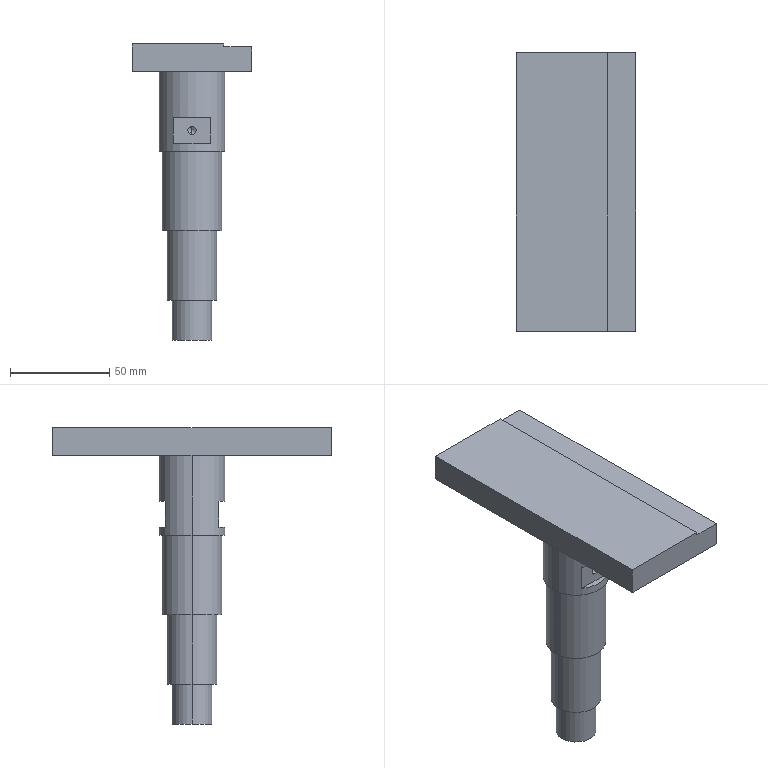Part | SolidWorks | features ICE 6, MirrorPattern 2, 3DProfileFeature 1, Extrusion 1, HoleWzd 1 | 1 solid | 34 faces | box 60 x 140 x 149 mm | volume 199315 mm3 | plane 18 | cylinder 12 | cone 4 | commonest cylinder face diameters 4.2 x4 20 x2 25 x2 30 x2 33 x2
STEP:
#1=CARTESIAN_POINT('',(0.,-3.5,52.6));
#2=VERTEX_POINT('',#1);
#3=CARTESIAN_POINT('',(0.,-3.5,48.4));
#4=VERTEX_POINT('',#3);
#5=CARTESIAN_POINT('',(0.,-3.5,50.5));
#6=DIRECTION('',(0.,-1.,0.));
#7=DIRECTION('',(0.,0.,-1.));
#8=AXIS2_PLACEMENT_3D('',#5,#6,#7);
#9=CIRCLE('',#8,2.1);
#10=EDGE_CURVE('',#2,#4,#9,.T.);
#11=ORIENTED_EDGE('',*,*,#10,.F.);
#12=CARTESIAN_POINT('',(0.,-13.5,52.6));
#13=VERTEX_POINT('',#12);
#14=CARTESIAN_POINT('',(0.,-13.5,52.6));
#15=DIRECTION('',(0.,-1.,0.));
#16=VECTOR('',#15,1000.);
#17=LINE('',#14,#16);
#18=EDGE_CURVE('',#2,#13,#17,.T.);
#19=ORIENTED_EDGE('',*,*,#18,.T.);
#20=CARTESIAN_POINT('',(0.,-13.5,48.4));
#21=VERTEX_POINT('',#20);
#22=CARTESIAN_POINT('',(0.,-13.5,50.5));
#23=DIRECTION('',(0.,-1.,0.));
#24=DIRECTION('',(0.,0.,-1.));
#25=AXIS2_PLACEMENT_3D('',#22,#23,#24);
#26=CIRCLE('',#25,2.1);
#27=EDGE_CURVE('',#13,#21,#26,.T.);
#28=ORIENTED_EDGE('',*,*,#27,.T.);
#29=CARTESIAN_POINT('',(0.,-13.5,48.4));
#30=DIRECTION('',(0.,-1.,0.));
#31=VECTOR('',#30,1000.);
#32=LINE('',#29,#31);
#33=EDGE_CURVE('',#4,#21,#32,.T.);
#34=ORIENTED_EDGE('',*,*,#33,.F.);
#35=EDGE_LOOP('',(#11,#19,#28,#34));
#36=FACE_OUTER_BOUND('',#35,.T.);
#37=CARTESIAN_POINT('',(0.,-13.5,50.5));
#38=DIRECTION('',(0.,-1.,0.));
#39=DIRECTION('',(0.,0.,-1.));
#40=AXIS2_PLACEMENT_3D('',#37,#38,#39);
#41=CYLINDRICAL_SURFACE('',#40,2.1);
#42=ADVANCED_FACE('',(#36),#41,.F.);
#43=CARTESIAN_POINT('',(0.,-2.238,50.5));
#44=VERTEX_POINT('',#43);
#45=CARTESIAN_POINT('',(0.,-3.5,48.4));
#46=DIRECTION('',(0.,-0.515,-0.8572));
#47=VECTOR('',#46,1000.);
#48=LINE('',#45,#47);
#49=EDGE_CURVE('',#44,#4,#48,.T.);
#50=ORIENTED_EDGE('',*,*,#49,.F.);
#51=CARTESIAN_POINT('',(0.,-3.5,52.6));
#52=DIRECTION('',(0.,-0.515,0.8572));
#53=VECTOR('',#52,1000.);
#54=LINE('',#51,#53);
#55=EDGE_CURVE('',#44,#2,#54,.T.);
#56=ORIENTED_EDGE('',*,*,#55,.T.);
#57=ORIENTED_EDGE('',*,*,#10,.T.);
#58=EDGE_LOOP('',(#50,#56,#57));
#59=FACE_OUTER_BOUND('',#58,.T.);
#60=CARTESIAN_POINT('',(0.,-3.5,50.5));
#61=DIRECTION('',(0.,-1.,0.));
#62=DIRECTION('',(0.,0.,-1.));
#63=AXIS2_PLACEMENT_3D('',#60,#61,#62);
#64=CONICAL_SURFACE('',#63,2.1,1.03);
#65=ADVANCED_FACE('',(#59),#64,.F.);
#66=CARTESIAN_POINT('',(0.,3.5,48.4));
#67=VERTEX_POINT('',#66);
#68=CARTESIAN_POINT('',(0.,3.5,52.6));
#69=VERTEX_POINT('',#68);
#70=CARTESIAN_POINT('',(0.,3.5,50.5));
#71=DIRECTION('',(0.,1.,0.));
#72=DIRECTION('',(0.,0.,1.));
#73=AXIS2_PLACEMENT_3D('',#70,#71,#72);
#74=CIRCLE('',#73,2.1);
#75=EDGE_CURVE('',#67,#69,#74,.T.);
#76=ORIENTED_EDGE('',*,*,#75,.F.);
#77=CARTESIAN_POINT('',(0.,13.5,48.4));
#78=VERTEX_POINT('',#77);
#79=CARTESIAN_POINT('',(0.,13.5,48.4));
#80=DIRECTION('',(0.,1.,0.));
#81=VECTOR('',#80,1000.);
#82=LINE('',#79,#81);
#83=EDGE_CURVE('',#67,#78,#82,.T.);
#84=ORIENTED_EDGE('',*,*,#83,.T.);
#85=CARTESIAN_POINT('',(0.,13.5,52.6));
#86=VERTEX_POINT('',#85);
#87=CARTESIAN_POINT('',(0.,13.5,50.5));
#88=DIRECTION('',(0.,1.,0.));
#89=DIRECTION('',(0.,0.,1.));
#90=AXIS2_PLACEMENT_3D('',#87,#88,#89);
#91=CIRCLE('',#90,2.1);
#92=EDGE_CURVE('',#78,#86,#91,.T.);
#93=ORIENTED_EDGE('',*,*,#92,.T.);
#94=CARTESIAN_POINT('',(0.,13.5,52.6));
#95=DIRECTION('',(0.,1.,0.));
#96=VECTOR('',#95,1000.);
#97=LINE('',#94,#96);
#98=EDGE_CURVE('',#69,#86,#97,.T.);
#99=ORIENTED_EDGE('',*,*,#98,.F.);
#100=EDGE_LOOP('',(#76,#84,#93,#99));
#101=FACE_OUTER_BOUND('',#100,.T.);
#102=CARTESIAN_POINT('',(0.,13.5,50.5));
#103=DIRECTION('',(0.,1.,0.));
#104=DIRECTION('',(0.,0.,1.));
#105=AXIS2_PLACEMENT_3D('',#102,#103,#104);
#106=CYLINDRICAL_SURFACE('',#105,2.1);
#107=ADVANCED_FACE('',(#101),#106,.F.);
#108=CARTESIAN_POINT('',(0.,2.238,50.5));
#109=VERTEX_POINT('',#108);
#110=CARTESIAN_POINT('',(0.,3.5,52.6));
#111=DIRECTION('',(0.,0.515,0.8572));
#112=VECTOR('',#111,1000.);
#113=LINE('',#110,#112);
#114=EDGE_CURVE('',#109,#69,#113,.T.);
#115=ORIENTED_EDGE('',*,*,#114,.F.);
#116=CARTESIAN_POINT('',(0.,3.5,48.4));
#117=DIRECTION('',(0.,0.515,-0.8572));
#118=VECTOR('',#117,1000.);
#119=LINE('',#116,#118);
#120=EDGE_CURVE('',#109,#67,#119,.T.);
#121=ORIENTED_EDGE('',*,*,#120,.T.);
#122=ORIENTED_EDGE('',*,*,#75,.T.);
#123=EDGE_LOOP('',(#115,#121,#122));
#124=FACE_OUTER_BOUND('',#123,.T.);
#125=CARTESIAN_POINT('',(0.,3.5,50.5));
#126=DIRECTION('',(0.,1.,0.));
#127=DIRECTION('',(0.,0.,1.));
#128=AXIS2_PLACEMENT_3D('',#125,#126,#127);
#129=CONICAL_SURFACE('',#128,2.1,1.03);
#130=ADVANCED_FACE('',(#124),#129,.F.);
#131=CARTESIAN_POINT('',(-10.,0.,-55.));
#132=VERTEX_POINT('',#131);
#133=CARTESIAN_POINT('',(10.,0.,-55.));
#134=VERTEX_POINT('',#133);
#135=CARTESIAN_POINT('',(0.,0.,-55.));
#136=DIRECTION('',(0.,0.,-1.));
#137=DIRECTION('',(-1.,0.,0.));
#138=AXIS2_PLACEMENT_3D('',#135,#136,#137);
#139=CIRCLE('',#138,10.);
#140=EDGE_CURVE('',#132,#134,#139,.T.);
#141=ORIENTED_EDGE('',*,*,#140,.F.);
#142=CARTESIAN_POINT('',(-10.,0.,-35.));
#143=VERTEX_POINT('',#142);
#144=CARTESIAN_POINT('',(-10.,0.,-55.));
#145=DIRECTION('',(0.,0.,1.));
#146=VECTOR('',#145,1000.);
#147=LINE('',#144,#146);
#148=EDGE_CURVE('',#132,#143,#147,.T.);
#149=ORIENTED_EDGE('',*,*,#148,.T.);
#150=CARTESIAN_POINT('',(10.,0.,-35.));
#151=VERTEX_POINT('',#150);
#152=CARTESIAN_POINT('',(0.,0.,-35.));
#153=DIRECTION('',(0.,0.,-1.));
#154=DIRECTION('',(-1.,0.,0.));
#155=AXIS2_PLACEMENT_3D('',#152,#153,#154);
#156=CIRCLE('',#155,10.);
#157=EDGE_CURVE('',#143,#151,#156,.T.);
#158=ORIENTED_EDGE('',*,*,#157,.T.);
#159=CARTESIAN_POINT('',(10.,0.,-55.));
#160=DIRECTION('',(0.,0.,1.));
#161=VECTOR('',#160,1000.);
#162=LINE('',#159,#161);
#163=EDGE_CURVE('',#134,#151,#162,.T.);
#164=ORIENTED_EDGE('',*,*,#163,.F.);
#165=EDGE_LOOP('',(#141,#149,#158,#164));
#166=FACE_OUTER_BOUND('',#165,.T.);
#167=CARTESIAN_POINT('',(0.,0.,-55.));
#168=DIRECTION('',(0.,0.,1.));
#169=DIRECTION('',(1.,0.,0.));
#170=AXIS2_PLACEMENT_3D('',#167,#168,#169);
#171=CYLINDRICAL_SURFACE('',#170,10.);
#172=ADVANCED_FACE('',(#166),#171,.T.);
#173=CARTESIAN_POINT('',(-12.5,0.,-35.));
#174=VERTEX_POINT('',#173);
#175=CARTESIAN_POINT('',(12.5,0.,-35.));
#176=VERTEX_POINT('',#175);
#177=CARTESIAN_POINT('',(0.,0.,-35.));
#178=DIRECTION('',(0.,0.,-1.));
#179=DIRECTION('',(-1.,0.,0.));
#180=AXIS2_PLACEMENT_3D('',#177,#178,#179);
#181=CIRCLE('',#180,12.5);
#182=EDGE_CURVE('',#174,#176,#181,.T.);
#183=ORIENTED_EDGE('',*,*,#182,.F.);
#184=CARTESIAN_POINT('',(-12.5,0.,0.));
#185=VERTEX_POINT('',#184);
#186=CARTESIAN_POINT('',(-12.5,0.,-35.));
#187=DIRECTION('',(0.,0.,1.));
#188=VECTOR('',#187,1000.);
#189=LINE('',#186,#188);
#190=EDGE_CURVE('',#174,#185,#189,.T.);
#191=ORIENTED_EDGE('',*,*,#190,.T.);
#192=CARTESIAN_POINT('',(12.5,0.,0.));
#193=VERTEX_POINT('',#192);
#194=CARTESIAN_POINT('',(0.,0.,0.));
#195=DIRECTION('',(0.,0.,-1.));
#196=DIRECTION('',(-1.,0.,0.));
#197=AXIS2_PLACEMENT_3D('',#194,#195,#196);
#198=CIRCLE('',#197,12.5);
#199=EDGE_CURVE('',#185,#193,#198,.T.);
#200=ORIENTED_EDGE('',*,*,#199,.T.);
#201=CARTESIAN_POINT('',(12.5,0.,-35.));
#202=DIRECTION('',(0.,0.,1.));
#203=VECTOR('',#202,1000.);
#204=LINE('',#201,#203);
#205=EDGE_CURVE('',#176,#193,#204,.T.);
#206=ORIENTED_EDGE('',*,*,#205,.F.);
#207=EDGE_LOOP('',(#183,#191,#200,#206));
#208=FACE_OUTER_BOUND('',#207,.T.);
#209=CARTESIAN_POINT('',(0.,0.,-35.));
#210=DIRECTION('',(0.,0.,1.));
#211=DIRECTION('',(1.,0.,0.));
#212=AXIS2_PLACEMENT_3D('',#209,#210,#211);
#213=CYLINDRICAL_SURFACE('',#212,12.5);
#214=ADVANCED_FACE('',(#208),#213,.T.);
#215=CARTESIAN_POINT('',(15.,0.,40.));
#216=VERTEX_POINT('',#215);
#217=CARTESIAN_POINT('',(-15.,0.,40.));
#218=VERTEX_POINT('',#217);
#219=CARTESIAN_POINT('',(0.,0.,40.));
#220=DIRECTION('',(0.,0.,1.));
#221=DIRECTION('',(1.,0.,0.));
#222=AXIS2_PLACEMENT_3D('',#219,#220,#221);
#223=CIRCLE('',#222,15.);
#224=EDGE_CURVE('',#216,#218,#223,.T.);
#225=ORIENTED_EDGE('',*,*,#224,.F.);
#226=CARTESIAN_POINT('',(15.,0.,0.));
#227=VERTEX_POINT('',#226);
#228=CARTESIAN_POINT('',(15.,0.,40.));
#229=DIRECTION('',(0.,0.,-1.));
#230=VECTOR('',#229,1000.);
#231=LINE('',#228,#230);
#232=EDGE_CURVE('',#216,#227,#231,.T.);
#233=ORIENTED_EDGE('',*,*,#232,.T.);
#234=CARTESIAN_POINT('',(-15.,0.,0.));
#235=VERTEX_POINT('',#234);
#236=CARTESIAN_POINT('',(0.,0.,0.));
#237=DIRECTION('',(0.,0.,1.));
#238=DIRECTION('',(1.,0.,0.));
#239=AXIS2_PLACEMENT_3D('',#236,#237,#238);
#240=CIRCLE('',#239,15.);
#241=EDGE_CURVE('',#227,#235,#240,.T.);
#242=ORIENTED_EDGE('',*,*,#241,.T.);
#243=CARTESIAN_POINT('',(-15.,0.,40.));
#244=DIRECTION('',(0.,0.,-1.));
#245=VECTOR('',#244,1000.);
#246=LINE('',#243,#245);
#247=EDGE_CURVE('',#218,#235,#246,.T.);
#248=ORIENTED_EDGE('',*,*,#247,.F.);
#249=EDGE_LOOP('',(#225,#233,#242,#248));
#250=FACE_OUTER_BOUND('',#249,.T.);
#251=CARTESIAN_POINT('',(0.,0.,40.));
#252=DIRECTION('',(0.,0.,-1.));
#253=DIRECTION('',(-1.,0.,0.));
#254=AXIS2_PLACEMENT_3D('',#251,#252,#253);
#255=CYLINDRICAL_SURFACE('',#254,15.);
#256=ADVANCED_FACE('',(#250),#255,.T.);
#257=CARTESIAN_POINT('',(-9.487,13.5,57.));
#258=VERTEX_POINT('',#257);
#259=CARTESIAN_POINT('',(-9.487,13.5,44.));
#260=VERTEX_POINT('',#259);
#261=CARTESIAN_POINT('',(-9.487,13.5,80.));
#262=DIRECTION('',(0.,0.,-1.));
#263=VECTOR('',#262,1000.);
#264=LINE('',#261,#263);
#265=EDGE_CURVE('',#258,#260,#264,.T.);
#266=ORIENTED_EDGE('',*,*,#265,.T.);
#267=CARTESIAN_POINT('',(9.487,13.5,44.));
#268=VERTEX_POINT('',#267);
#269=CARTESIAN_POINT('',(0.,0.,44.));
#270=DIRECTION('',(0.,0.,-1.));
#271=DIRECTION('',(-1.,0.,0.));
#272=AXIS2_PLACEMENT_3D('',#269,#270,#271);
#273=CIRCLE('',#272,16.5);
#274=EDGE_CURVE('',#260,#268,#273,.T.);
#275=ORIENTED_EDGE('',*,*,#274,.T.);
#276=CARTESIAN_POINT('',(9.487,13.5,57.));
#277=VERTEX_POINT('',#276);
#278=CARTESIAN_POINT('',(9.487,13.5,80.));
#279=DIRECTION('',(0.,0.,1.));
#280=VECTOR('',#279,1000.);
#281=LINE('',#278,#280);
#282=EDGE_CURVE('',#268,#277,#281,.T.);
#283=ORIENTED_EDGE('',*,*,#282,.T.);
#284=CARTESIAN_POINT('',(0.,0.,57.));
#285=DIRECTION('',(0.,0.,1.));
#286=DIRECTION('',(1.,0.,0.));
#287=AXIS2_PLACEMENT_3D('',#284,#285,#286);
#288=CIRCLE('',#287,16.5);
#289=EDGE_CURVE('',#277,#258,#288,.T.);
#290=ORIENTED_EDGE('',*,*,#289,.T.);
#291=EDGE_LOOP('',(#266,#275,#283,#290));
#292=FACE_BOUND('',#291,.T.);
#293=CARTESIAN_POINT('',(16.5,0.,80.));
#294=VERTEX_POINT('',#293);
#295=CARTESIAN_POINT('',(-16.5,0.,80.));
#296=VERTEX_POINT('',#295);
#297=CARTESIAN_POINT('',(0.,0.,80.));
#298=DIRECTION('',(0.,0.,1.));
#299=DIRECTION('',(1.,0.,0.));
#300=AXIS2_PLACEMENT_3D('',#297,#298,#299);
#301=CIRCLE('',#300,16.5);
#302=EDGE_CURVE('',#294,#296,#301,.T.);
#303=ORIENTED_EDGE('',*,*,#302,.F.);
#304=CARTESIAN_POINT('',(16.5,0.,40.));
#305=VERTEX_POINT('',#304);
#306=CARTESIAN_POINT('',(16.5,0.,80.));
#307=DIRECTION('',(0.,0.,-1.));
#308=VECTOR('',#307,1000.);
#309=LINE('',#306,#308);
#310=EDGE_CURVE('',#294,#305,#309,.T.);
#311=ORIENTED_EDGE('',*,*,#310,.T.);
#312=CARTESIAN_POINT('',(-16.5,0.,40.));
#313=VERTEX_POINT('',#312);
#314=CARTESIAN_POINT('',(0.,0.,40.));
#315=DIRECTION('',(0.,0.,1.));
#316=DIRECTION('',(1.,0.,0.));
#317=AXIS2_PLACEMENT_3D('',#314,#315,#316);
#318=CIRCLE('',#317,16.5);
#319=EDGE_CURVE('',#305,#313,#318,.T.);
#320=ORIENTED_EDGE('',*,*,#319,.T.);
#321=CARTESIAN_POINT('',(-16.5,0.,80.));
#322=DIRECTION('',(0.,0.,-1.));
#323=VECTOR('',#322,1000.);
#324=LINE('',#321,#323);
#325=EDGE_CURVE('',#296,#313,#324,.T.);
#326=ORIENTED_EDGE('',*,*,#325,.F.);
#327=EDGE_LOOP('',(#303,#311,#320,#326));
#328=FACE_OUTER_BOUND('',#327,.T.);
#329=CARTESIAN_POINT('',(0.,0.,80.));
#330=DIRECTION('',(0.,0.,-1.));
#331=DIRECTION('',(-1.,0.,0.));
#332=AXIS2_PLACEMENT_3D('',#329,#330,#331);
#333=CYLINDRICAL_SURFACE('',#332,16.5);
#334=ADVANCED_FACE('',(#292,#328),#333,.T.);
#335=ORIENTED_EDGE('',*,*,#310,.F.);
#336=CARTESIAN_POINT('',(0.,0.,80.));
#337=DIRECTION('',(0.,0.,1.));
#338=DIRECTION('',(1.,0.,0.));
#339=AXIS2_PLACEMENT_3D('',#336,#337,#338);
#340=CIRCLE('',#339,16.5);
#341=EDGE_CURVE('',#296,#294,#340,.T.);
#342=ORIENTED_EDGE('',*,*,#341,.F.);
#343=ORIENTED_EDGE('',*,*,#325,.T.);
#344=CARTESIAN_POINT('',(0.,0.,40.));
#345=DIRECTION('',(0.,0.,1.));
#346=DIRECTION('',(1.,0.,0.));
#347=AXIS2_PLACEMENT_3D('',#344,#345,#346);
#348=CIRCLE('',#347,16.5);
#349=EDGE_CURVE('',#313,#305,#348,.T.);
#350=ORIENTED_EDGE('',*,*,#349,.T.);
#351=EDGE_LOOP('',(#335,#342,#343,#350));
#352=FACE_OUTER_BOUND('',#351,.T.);
#353=CARTESIAN_POINT('',(9.487,-13.5,57.));
#354=VERTEX_POINT('',#353);
#355=CARTESIAN_POINT('',(-9.487,-13.5,57.));
#356=VERTEX_POINT('',#355);
#357=CARTESIAN_POINT('',(0.,0.,57.));
#358=DIRECTION('',(0.,0.,-1.));
#359=DIRECTION('',(-1.,0.,0.));
#360=AXIS2_PLACEMENT_3D('',#357,#358,#359);
#361=CIRCLE('',#360,16.5);
#362=EDGE_CURVE('',#354,#356,#361,.T.);
#363=ORIENTED_EDGE('',*,*,#362,.F.);
#364=CARTESIAN_POINT('',(9.487,-13.5,44.));
#365=VERTEX_POINT('',#364);
#366=CARTESIAN_POINT('',(9.487,-13.5,80.));
#367=DIRECTION('',(0.,0.,1.));
#368=VECTOR('',#367,1000.);
#369=LINE('',#366,#368);
#370=EDGE_CURVE('',#365,#354,#369,.T.);
#371=ORIENTED_EDGE('',*,*,#370,.F.);
#372=CARTESIAN_POINT('',(-9.487,-13.5,44.));
#373=VERTEX_POINT('',#372);
#374=CARTESIAN_POINT('',(0.,0.,44.));
#375=DIRECTION('',(0.,0.,1.));
#376=DIRECTION('',(1.,0.,0.));
#377=AXIS2_PLACEMENT_3D('',#374,#375,#376);
#378=CIRCLE('',#377,16.5);
#379=EDGE_CURVE('',#373,#365,#378,.T.);
#380=ORIENTED_EDGE('',*,*,#379,.F.);
#381=CARTESIAN_POINT('',(-9.487,-13.5,80.));
#382=DIRECTION('',(0.,0.,-1.));
#383=VECTOR('',#382,1000.);
#384=LINE('',#381,#383);
#385=EDGE_CURVE('',#356,#373,#384,.T.);
#386=ORIENTED_EDGE('',*,*,#385,.F.);
#387=EDGE_LOOP('',(#363,#371,#380,#386));
#388=FACE_BOUND('',#387,.T.);
#389=CARTESIAN_POINT('',(0.,0.,80.));
#390=DIRECTION('',(0.,0.,-1.));
#391=DIRECTION('',(-1.,0.,0.));
#392=AXIS2_PLACEMENT_3D('',#389,#390,#391);
#393=CYLINDRICAL_SURFACE('',#392,16.5);
#394=ADVANCED_FACE('',(#352,#388),#393,.T.);
#395=ORIENTED_EDGE('',*,*,#232,.F.);
#396=CARTESIAN_POINT('',(0.,0.,40.));
#397=DIRECTION('',(0.,0.,1.));
#398=DIRECTION('',(1.,0.,0.));
#399=AXIS2_PLACEMENT_3D('',#396,#397,#398);
#400=CIRCLE('',#399,15.);
#401=EDGE_CURVE('',#218,#216,#400,.T.);
#402=ORIENTED_EDGE('',*,*,#401,.F.);
#403=ORIENTED_EDGE('',*,*,#247,.T.);
#404=CARTESIAN_POINT('',(0.,0.,0.));
#405=DIRECTION('',(0.,0.,1.));
#406=DIRECTION('',(1.,0.,0.));
#407=AXIS2_PLACEMENT_3D('',#404,#405,#406);
#408=CIRCLE('',#407,15.);
#409=EDGE_CURVE('',#235,#227,#408,.T.);
#410=ORIENTED_EDGE('',*,*,#409,.T.);
#411=EDGE_LOOP('',(#395,#402,#403,#410));
#412=FACE_OUTER_BOUND('',#411,.T.);
#413=CARTESIAN_POINT('',(0.,0.,40.));
#414=DIRECTION('',(0.,0.,-1.));
#415=DIRECTION('',(-1.,0.,0.));
#416=AXIS2_PLACEMENT_3D('',#413,#414,#415);
#417=CYLINDRICAL_SURFACE('',#416,15.);
#418=ADVANCED_FACE('',(#412),#417,.T.);
#419=CARTESIAN_POINT('',(0.,0.,0.));
#420=DIRECTION('',(0.,0.,-1.));
#421=DIRECTION('',(-1.,0.,0.));
#422=AXIS2_PLACEMENT_3D('',#419,#420,#421);
#423=CIRCLE('',#422,12.5);
#424=EDGE_CURVE('',#193,#185,#423,.T.);
#425=ORIENTED_EDGE('',*,*,#424,.F.);
#426=ORIENTED_EDGE('',*,*,#199,.F.);
#427=EDGE_LOOP('',(#425,#426));
#428=FACE_BOUND('',#427,.T.);
#429=ORIENTED_EDGE('',*,*,#409,.F.);
#430=ORIENTED_EDGE('',*,*,#241,.F.);
#431=EDGE_LOOP('',(#429,#430));
#432=FACE_OUTER_BOUND('',#431,.T.);
#433=CARTESIAN_POINT('',(0.,0.,0.));
#434=DIRECTION('',(0.,0.,1.));
#435=DIRECTION('',(1.,0.,0.));
#436=AXIS2_PLACEMENT_3D('',#433,#434,#435);
#437=PLANE('',#436);
#438=ADVANCED_FACE('',(#428,#432),#437,.F.);
#439=ORIENTED_EDGE('',*,*,#401,.T.);
#440=ORIENTED_EDGE('',*,*,#224,.T.);
#441=EDGE_LOOP('',(#439,#440));
#442=FACE_BOUND('',#441,.T.);
#443=ORIENTED_EDGE('',*,*,#349,.F.);
#444=ORIENTED_EDGE('',*,*,#319,.F.);
#445=EDGE_LOOP('',(#443,#444));
#446=FACE_OUTER_BOUND('',#445,.T.);
#447=CARTESIAN_POINT('',(0.,0.,40.));
#448=DIRECTION('',(0.,0.,1.));
#449=DIRECTION('',(1.,0.,0.));
#450=AXIS2_PLACEMENT_3D('',#447,#448,#449);
#451=PLANE('',#450);
#452=ADVANCED_FACE('',(#442,#446),#451,.F.);
#453=ORIENTED_EDGE('',*,*,#190,.F.);
#454=CARTESIAN_POINT('',(0.,0.,-35.));
#455=DIRECTION('',(0.,0.,-1.));
#456=DIRECTION('',(-1.,0.,0.));
#457=AXIS2_PLACEMENT_3D('',#454,#455,#456);
#458=CIRCLE('',#457,12.5);
#459=EDGE_CURVE('',#176,#174,#458,.T.);
#460=ORIENTED_EDGE('',*,*,#459,.F.);
#461=ORIENTED_EDGE('',*,*,#205,.T.);
#462=ORIENTED_EDGE('',*,*,#424,.T.);
#463=EDGE_LOOP('',(#453,#460,#461,#462));
#464=FACE_OUTER_BOUND('',#463,.T.);
#465=CARTESIAN_POINT('',(0.,0.,-35.));
#466=DIRECTION('',(0.,0.,1.));
#467=DIRECTION('',(1.,0.,0.));
#468=AXIS2_PLACEMENT_3D('',#465,#466,#467);
#469=CYLINDRICAL_SURFACE('',#468,12.5);
#470=ADVANCED_FACE('',(#464),#469,.T.);
#471=CARTESIAN_POINT('',(0.,0.,-35.));
#472=DIRECTION('',(0.,0.,-1.));
#473=DIRECTION('',(-1.,0.,0.));
#474=AXIS2_PLACEMENT_3D('',#471,#472,#473);
#475=CIRCLE('',#474,10.);
#476=EDGE_CURVE('',#151,#143,#475,.T.);
#477=ORIENTED_EDGE('',*,*,#476,.F.);
#478=ORIENTED_EDGE('',*,*,#157,.F.);
#479=EDGE_LOOP('',(#477,#478));
#480=FACE_BOUND('',#479,.T.);
#481=ORIENTED_EDGE('',*,*,#459,.T.);
#482=ORIENTED_EDGE('',*,*,#182,.T.);
#483=EDGE_LOOP('',(#481,#482));
#484=FACE_OUTER_BOUND('',#483,.T.);
#485=CARTESIAN_POINT('',(0.,0.,-35.));
#486=DIRECTION('',(0.,0.,-1.));
#487=DIRECTION('',(-1.,0.,0.));
#488=AXIS2_PLACEMENT_3D('',#485,#486,#487);
#489=PLANE('',#488);
#490=ADVANCED_FACE('',(#480,#484),#489,.T.);
#491=ORIENTED_EDGE('',*,*,#148,.F.);
#492=CARTESIAN_POINT('',(0.,0.,-55.));
#493=DIRECTION('',(0.,0.,-1.));
#494=DIRECTION('',(-1.,0.,0.));
#495=AXIS2_PLACEMENT_3D('',#492,#493,#494);
#496=CIRCLE('',#495,10.);
#497=EDGE_CURVE('',#134,#132,#496,.T.);
#498=ORIENTED_EDGE('',*,*,#497,.F.);
#499=ORIENTED_EDGE('',*,*,#163,.T.);
#500=ORIENTED_EDGE('',*,*,#476,.T.);
#501=EDGE_LOOP('',(#491,#498,#499,#500));
#502=FACE_OUTER_BOUND('',#501,.T.);
#503=CARTESIAN_POINT('',(0.,0.,-55.));
#504=DIRECTION('',(0.,0.,1.));
#505=DIRECTION('',(1.,0.,0.));
#506=AXIS2_PLACEMENT_3D('',#503,#504,#505);
#507=CYLINDRICAL_SURFACE('',#506,10.);
#508=ADVANCED_FACE('',(#502),#507,.T.);
#509=ORIENTED_EDGE('',*,*,#497,.T.);
#510=ORIENTED_EDGE('',*,*,#140,.T.);
#511=EDGE_LOOP('',(#509,#510));
#512=FACE_OUTER_BOUND('',#511,.T.);
#513=CARTESIAN_POINT('',(0.,0.,-55.));
#514=DIRECTION('',(0.,0.,-1.));
#515=DIRECTION('',(-1.,0.,0.));
#516=AXIS2_PLACEMENT_3D('',#513,#514,#515);
#517=PLANE('',#516);
#518=ADVANCED_FACE('',(#512),#517,.T.);
#519=CARTESIAN_POINT('',(30.,70.,92.5));
#520=VERTEX_POINT('',#519);
#521=CARTESIAN_POINT('',(30.,70.,80.));
#522=VERTEX_POINT('',#521);
#523=CARTESIAN_POINT('',(30.,70.,94.));
#524=DIRECTION('',(0.,0.,-1.));
#525=VECTOR('',#524,1000.);
#526=LINE('',#523,#525);
#527=EDGE_CURVE('',#520,#522,#526,.T.);
#528=ORIENTED_EDGE('',*,*,#527,.F.);
#529=CARTESIAN_POINT('',(30.,-70.,92.5));
#530=VERTEX_POINT('',#529);
#531=CARTESIAN_POINT('',(30.,70.,92.5));
#532=DIRECTION('',(0.,1.,0.));
#533=VECTOR('',#532,1000.);
#534=LINE('',#531,#533);
#535=EDGE_CURVE('',#530,#520,#534,.T.);
#536=ORIENTED_EDGE('',*,*,#535,.F.);
#537=CARTESIAN_POINT('',(30.,-70.,80.));
#538=VERTEX_POINT('',#537);
#539=CARTESIAN_POINT('',(30.,-70.,94.));
#540=DIRECTION('',(0.,0.,-1.));
#541=VECTOR('',#540,1000.);
#542=LINE('',#539,#541);
#543=EDGE_CURVE('',#530,#538,#542,.T.);
#544=ORIENTED_EDGE('',*,*,#543,.T.);
#545=CARTESIAN_POINT('',(30.,-70.,80.));
#546=DIRECTION('',(0.,1.,0.));
#547=VECTOR('',#546,1000.);
#548=LINE('',#545,#547);
#549=EDGE_CURVE('',#538,#522,#548,.T.);
#550=ORIENTED_EDGE('',*,*,#549,.T.);
#551=EDGE_LOOP('',(#528,#536,#544,#550));
#552=FACE_OUTER_BOUND('',#551,.T.);
#553=CARTESIAN_POINT('',(30.,-70.,94.));
#554=DIRECTION('',(-1.,0.,0.));
#555=DIRECTION('',(0.,0.,1.));
#556=AXIS2_PLACEMENT_3D('',#553,#554,#555);
#557=PLANE('',#556);
#558=ADVANCED_FACE('',(#552),#557,.F.);
#559=CARTESIAN_POINT('',(16.,70.,94.));
#560=VERTEX_POINT('',#559);
#561=CARTESIAN_POINT('',(-30.,70.,94.));
#562=VERTEX_POINT('',#561);
#563=CARTESIAN_POINT('',(-30.,70.,94.));
#564=DIRECTION('',(-1.,0.,0.));
#565=VECTOR('',#564,1000.);
#566=LINE('',#563,#565);
#567=EDGE_CURVE('',#560,#562,#566,.T.);
#568=ORIENTED_EDGE('',*,*,#567,.F.);
#569=CARTESIAN_POINT('',(16.,70.,92.5));
#570=VERTEX_POINT('',#569);
#571=CARTESIAN_POINT('',(16.,70.,92.5));
#572=DIRECTION('',(0.,0.,1.));
#573=VECTOR('',#572,1000.);
#574=LINE('',#571,#573);
#575=EDGE_CURVE('',#570,#560,#574,.T.);
#576=ORIENTED_EDGE('',*,*,#575,.F.);
#577=CARTESIAN_POINT('',(30.,70.,92.5));
#578=DIRECTION('',(-1.,0.,0.));
#579=VECTOR('',#578,1000.);
#580=LINE('',#577,#579);
#581=EDGE_CURVE('',#520,#570,#580,.T.);
#582=ORIENTED_EDGE('',*,*,#581,.F.);
#583=ORIENTED_EDGE('',*,*,#527,.T.);
#584=CARTESIAN_POINT('',(-30.,70.,80.));
#585=VERTEX_POINT('',#584);
#586=CARTESIAN_POINT('',(-30.,70.,80.));
#587=DIRECTION('',(-1.,0.,0.));
#588=VECTOR('',#587,1000.);
#589=LINE('',#586,#588);
#590=EDGE_CURVE('',#522,#585,#589,.T.);
#591=ORIENTED_EDGE('',*,*,#590,.T.);
#592=CARTESIAN_POINT('',(-30.,70.,94.));
#593=DIRECTION('',(0.,0.,-1.));
#594=VECTOR('',#593,1000.);
#595=LINE('',#592,#594);
#596=EDGE_CURVE('',#562,#585,#595,.T.);
#597=ORIENTED_EDGE('',*,*,#596,.F.);
#598=EDGE_LOOP('',(#568,#576,#582,#583,#591,#597));
#599=FACE_OUTER_BOUND('',#598,.T.);
#600=CARTESIAN_POINT('',(-30.,70.,94.));
#601=DIRECTION('',(0.,-1.,0.));
#602=DIRECTION('',(0.,0.,-1.));
#603=AXIS2_PLACEMENT_3D('',#600,#601,#602);
#604=PLANE('',#603);
#605=ADVANCED_FACE('',(#599),#604,.F.);
#606=CARTESIAN_POINT('',(-30.,-70.,80.));
#607=VERTEX_POINT('',#606);
#608=CARTESIAN_POINT('',(-30.,-70.,80.));
#609=DIRECTION('',(0.,-1.,0.));
#610=VECTOR('',#609,1000.);
#611=LINE('',#608,#610);
#612=EDGE_CURVE('',#585,#607,#611,.T.);
#613=ORIENTED_EDGE('',*,*,#612,.T.);
#614=CARTESIAN_POINT('',(-30.,-70.,94.));
#615=VERTEX_POINT('',#614);
#616=CARTESIAN_POINT('',(-30.,-70.,94.));
#617=DIRECTION('',(0.,0.,-1.));
#618=VECTOR('',#617,1000.);
#619=LINE('',#616,#618);
#620=EDGE_CURVE('',#615,#607,#619,.T.);
#621=ORIENTED_EDGE('',*,*,#620,.F.);
#622=CARTESIAN_POINT('',(-30.,-70.,94.));
#623=DIRECTION('',(0.,-1.,0.));
#624=VECTOR('',#623,1000.);
#625=LINE('',#622,#624);
#626=EDGE_CURVE('',#562,#615,#625,.T.);
#627=ORIENTED_EDGE('',*,*,#626,.F.);
#628=ORIENTED_EDGE('',*,*,#596,.T.);
#629=EDGE_LOOP('',(#613,#621,#627,#628));
#630=FACE_OUTER_BOUND('',#629,.T.);
#631=CARTESIAN_POINT('',(-30.,-70.,94.));
#632=DIRECTION('',(1.,0.,0.));
#633=DIRECTION('',(0.,0.,-1.));
#634=AXIS2_PLACEMENT_3D('',#631,#632,#633);
#635=PLANE('',#634);
#636=ADVANCED_FACE('',(#630),#635,.F.);
#637=CARTESIAN_POINT('',(16.,-70.,92.5));
#638=VERTEX_POINT('',#637);
#639=CARTESIAN_POINT('',(30.,-70.,92.5));
#640=DIRECTION('',(1.,0.,0.));
#641=VECTOR('',#640,1000.);
#642=LINE('',#639,#641);
#643=EDGE_CURVE('',#638,#530,#642,.T.);
#644=ORIENTED_EDGE('',*,*,#643,.F.);
#645=CARTESIAN_POINT('',(16.,-70.,94.));
#646=VERTEX_POINT('',#645);
#647=CARTESIAN_POINT('',(16.,-70.,92.5));
#648=DIRECTION('',(0.,0.,1.));
#649=VECTOR('',#648,1000.);
#650=LINE('',#647,#649);
#651=EDGE_CURVE('',#638,#646,#650,.T.);
#652=ORIENTED_EDGE('',*,*,#651,.T.);
#653=CARTESIAN_POINT('',(-30.,-70.,94.));
#654=DIRECTION('',(1.,0.,0.));
#655=VECTOR('',#654,1000.);
#656=LINE('',#653,#655);
#657=EDGE_CURVE('',#615,#646,#656,.T.);
#658=ORIENTED_EDGE('',*,*,#657,.F.);
#659=ORIENTED_EDGE('',*,*,#620,.T.);
#660=CARTESIAN_POINT('',(-30.,-70.,80.));
#661=DIRECTION('',(1.,0.,0.));
#662=VECTOR('',#661,1000.);
#663=LINE('',#660,#662);
#664=EDGE_CURVE('',#607,#538,#663,.T.);
#665=ORIENTED_EDGE('',*,*,#664,.T.);
#666=ORIENTED_EDGE('',*,*,#543,.F.);
#667=EDGE_LOOP('',(#644,#652,#658,#659,#665,#666));
#668=FACE_OUTER_BOUND('',#667,.T.);
#669=CARTESIAN_POINT('',(-30.,-70.,94.));
#670=DIRECTION('',(0.,1.,0.));
#671=DIRECTION('',(0.,0.,1.));
#672=AXIS2_PLACEMENT_3D('',#669,#670,#671);
#673=PLANE('',#672);
#674=ADVANCED_FACE('',(#668),#673,.F.);
#675=ORIENTED_EDGE('',*,*,#657,.T.);
#676=CARTESIAN_POINT('',(16.,70.,94.));
#677=DIRECTION('',(0.,-1.,0.));
#678=VECTOR('',#677,1000.);
#679=LINE('',#676,#678);
#680=EDGE_CURVE('',#560,#646,#679,.T.);
#681=ORIENTED_EDGE('',*,*,#680,.F.);
#682=ORIENTED_EDGE('',*,*,#567,.T.);
#683=ORIENTED_EDGE('',*,*,#626,.T.);
#684=EDGE_LOOP('',(#675,#681,#682,#683));
#685=FACE_OUTER_BOUND('',#684,.T.);
#686=CARTESIAN_POINT('',(0.,0.,94.));
#687=DIRECTION('',(0.,0.,-1.));
#688=DIRECTION('',(-1.,0.,0.));
#689=AXIS2_PLACEMENT_3D('',#686,#687,#688);
#690=PLANE('',#689);
#691=ADVANCED_FACE('',(#685),#690,.F.);
#692=ORIENTED_EDGE('',*,*,#341,.T.);
#693=ORIENTED_EDGE('',*,*,#302,.T.);
#694=EDGE_LOOP('',(#692,#693));
#695=FACE_BOUND('',#694,.T.);
#696=ORIENTED_EDGE('',*,*,#549,.F.);
#697=ORIENTED_EDGE('',*,*,#664,.F.);
#698=ORIENTED_EDGE('',*,*,#612,.F.);
#699=ORIENTED_EDGE('',*,*,#590,.F.);
#700=EDGE_LOOP('',(#696,#697,#698,#699));
#701=FACE_OUTER_BOUND('',#700,.T.);
#702=CARTESIAN_POINT('',(0.,0.,80.));
#703=DIRECTION('',(0.,0.,-1.));
#704=DIRECTION('',(-1.,0.,0.));
#705=AXIS2_PLACEMENT_3D('',#702,#703,#704);
#706=PLANE('',#705);
#707=ADVANCED_FACE('',(#695,#701),#706,.T.);
#708=ORIENTED_EDGE('',*,*,#680,.T.);
#709=ORIENTED_EDGE('',*,*,#651,.F.);
#710=CARTESIAN_POINT('',(16.,70.,92.5));
#711=DIRECTION('',(0.,-1.,0.));
#712=VECTOR('',#711,1000.);
#713=LINE('',#710,#712);
#714=EDGE_CURVE('',#570,#638,#713,.T.);
#715=ORIENTED_EDGE('',*,*,#714,.F.);
#716=ORIENTED_EDGE('',*,*,#575,.T.);
#717=EDGE_LOOP('',(#708,#709,#715,#716));
#718=FACE_OUTER_BOUND('',#717,.T.);
#719=CARTESIAN_POINT('',(16.,70.,92.5));
#720=DIRECTION('',(-1.,0.,0.));
#721=DIRECTION('',(0.,-1.,0.));
#722=AXIS2_PLACEMENT_3D('',#719,#720,#721);
#723=PLANE('',#722);
#724=ADVANCED_FACE('',(#718),#723,.F.);
#725=ORIENTED_EDGE('',*,*,#535,.T.);
#726=ORIENTED_EDGE('',*,*,#581,.T.);
#727=ORIENTED_EDGE('',*,*,#714,.T.);
#728=ORIENTED_EDGE('',*,*,#643,.T.);
#729=EDGE_LOOP('',(#725,#726,#727,#728));
#730=FACE_OUTER_BOUND('',#729,.T.);
#731=CARTESIAN_POINT('',(0.,0.,92.5));
#732=DIRECTION('',(0.,0.,-1.));
#733=DIRECTION('',(-1.,0.,0.));
#734=AXIS2_PLACEMENT_3D('',#731,#732,#733);
#735=PLANE('',#734);
#736=ADVANCED_FACE('',(#730),#735,.F.);
#737=CARTESIAN_POINT('',(-10.,13.5,44.));
#738=DIRECTION('',(1.,0.,0.));
#739=VECTOR('',#738,1000.);
#740=LINE('',#737,#739);
#741=EDGE_CURVE('',#260,#268,#740,.T.);
#742=ORIENTED_EDGE('',*,*,#741,.T.);
#743=ORIENTED_EDGE('',*,*,#274,.F.);
#744=EDGE_LOOP('',(#742,#743));
#745=FACE_OUTER_BOUND('',#744,.T.);
#746=CARTESIAN_POINT('',(-10.,13.5,44.));
#747=DIRECTION('',(0.,0.,-1.));
#748=DIRECTION('',(-1.,0.,0.));
#749=AXIS2_PLACEMENT_3D('',#746,#747,#748);
#750=PLANE('',#749);
#751=ADVANCED_FACE('',(#745),#750,.F.);
#752=CARTESIAN_POINT('',(0.,13.5,50.5));
#753=DIRECTION('',(0.,1.,0.));
#754=DIRECTION('',(0.,0.,1.));
#755=AXIS2_PLACEMENT_3D('',#752,#753,#754);
#756=CIRCLE('',#755,2.1);
#757=EDGE_CURVE('',#86,#78,#756,.T.);
#758=ORIENTED_EDGE('',*,*,#757,.F.);
#759=ORIENTED_EDGE('',*,*,#92,.F.);
#760=EDGE_LOOP('',(#758,#759));
#761=FACE_BOUND('',#760,.T.);
#762=CARTESIAN_POINT('',(-10.,13.5,57.));
#763=DIRECTION('',(1.,0.,0.));
#764=VECTOR('',#763,1000.);
#765=LINE('',#762,#764);
#766=EDGE_CURVE('',#258,#277,#765,.T.);
#767=ORIENTED_EDGE('',*,*,#766,.T.);
#768=ORIENTED_EDGE('',*,*,#282,.F.);
#769=ORIENTED_EDGE('',*,*,#741,.F.);
#770=ORIENTED_EDGE('',*,*,#265,.F.);
#771=EDGE_LOOP('',(#767,#768,#769,#770));
#772=FACE_OUTER_BOUND('',#771,.T.);
#773=CARTESIAN_POINT('',(-10.,13.5,57.));
#774=DIRECTION('',(0.,-1.,0.));
#775=DIRECTION('',(0.,0.,-1.));
#776=AXIS2_PLACEMENT_3D('',#773,#774,#775);
#777=PLANE('',#776);
#778=ADVANCED_FACE('',(#761,#772),#777,.F.);
#779=ORIENTED_EDGE('',*,*,#766,.F.);
#780=ORIENTED_EDGE('',*,*,#289,.F.);
#781=EDGE_LOOP('',(#779,#780));
#782=FACE_OUTER_BOUND('',#781,.T.);
#783=CARTESIAN_POINT('',(-10.,16.5,57.));
#784=DIRECTION('',(0.,0.,1.));
#785=DIRECTION('',(1.,0.,0.));
#786=AXIS2_PLACEMENT_3D('',#783,#784,#785);
#787=PLANE('',#786);
#788=ADVANCED_FACE('',(#782),#787,.F.);
#789=CARTESIAN_POINT('',(-10.,-13.5,57.));
#790=DIRECTION('',(1.,0.,0.));
#791=VECTOR('',#790,1000.);
#792=LINE('',#789,#791);
#793=EDGE_CURVE('',#356,#354,#792,.T.);
#794=ORIENTED_EDGE('',*,*,#793,.T.);
#795=ORIENTED_EDGE('',*,*,#362,.T.);
#796=EDGE_LOOP('',(#794,#795));
#797=FACE_OUTER_BOUND('',#796,.T.);
#798=CARTESIAN_POINT('',(-10.,-16.5,57.));
#799=DIRECTION('',(0.,0.,-1.));
#800=DIRECTION('',(-1.,0.,0.));
#801=AXIS2_PLACEMENT_3D('',#798,#799,#800);
#802=PLANE('',#801);
#803=ADVANCED_FACE('',(#797),#802,.T.);
#804=CARTESIAN_POINT('',(0.,-13.5,50.5));
#805=DIRECTION('',(0.,-1.,0.));
#806=DIRECTION('',(0.,0.,-1.));
#807=AXIS2_PLACEMENT_3D('',#804,#805,#806);
#808=CIRCLE('',#807,2.1);
#809=EDGE_CURVE('',#21,#13,#808,.T.);
#810=ORIENTED_EDGE('',*,*,#809,.F.);
#811=ORIENTED_EDGE('',*,*,#27,.F.);
#812=EDGE_LOOP('',(#810,#811));
#813=FACE_BOUND('',#812,.T.);
#814=ORIENTED_EDGE('',*,*,#385,.T.);
#815=CARTESIAN_POINT('',(-10.,-13.5,44.));
#816=DIRECTION('',(1.,0.,0.));
#817=VECTOR('',#816,1000.);
#818=LINE('',#815,#817);
#819=EDGE_CURVE('',#373,#365,#818,.T.);
#820=ORIENTED_EDGE('',*,*,#819,.T.);
#821=ORIENTED_EDGE('',*,*,#370,.T.);
#822=ORIENTED_EDGE('',*,*,#793,.F.);
#823=EDGE_LOOP('',(#814,#820,#821,#822));
#824=FACE_OUTER_BOUND('',#823,.T.);
#825=CARTESIAN_POINT('',(-10.,-13.5,57.));
#826=DIRECTION('',(0.,-1.,0.));
#827=DIRECTION('',(0.,0.,-1.));
#828=AXIS2_PLACEMENT_3D('',#825,#826,#827);
#829=PLANE('',#828);
#830=ADVANCED_FACE('',(#813,#824),#829,.T.);
#831=ORIENTED_EDGE('',*,*,#819,.F.);
#832=ORIENTED_EDGE('',*,*,#379,.T.);
#833=EDGE_LOOP('',(#831,#832));
#834=FACE_OUTER_BOUND('',#833,.T.);
#835=CARTESIAN_POINT('',(-10.,-13.5,44.));
#836=DIRECTION('',(0.,0.,1.));
#837=DIRECTION('',(1.,0.,0.));
#838=AXIS2_PLACEMENT_3D('',#835,#836,#837);
#839=PLANE('',#838);
#840=ADVANCED_FACE('',(#834),#839,.T.);
#841=ORIENTED_EDGE('',*,*,#120,.F.);
#842=ORIENTED_EDGE('',*,*,#114,.T.);
#843=CARTESIAN_POINT('',(0.,3.5,50.5));
#844=DIRECTION('',(0.,1.,0.));
#845=DIRECTION('',(0.,0.,1.));
#846=AXIS2_PLACEMENT_3D('',#843,#844,#845);
#847=CIRCLE('',#846,2.1);
#848=EDGE_CURVE('',#69,#67,#847,.T.);
#849=ORIENTED_EDGE('',*,*,#848,.T.);
#850=EDGE_LOOP('',(#841,#842,#849));
#851=FACE_OUTER_BOUND('',#850,.T.);
#852=CARTESIAN_POINT('',(0.,3.5,50.5));
#853=DIRECTION('',(0.,1.,0.));
#854=DIRECTION('',(0.,0.,1.));
#855=AXIS2_PLACEMENT_3D('',#852,#853,#854);
#856=CONICAL_SURFACE('',#855,2.1,1.03);
#857=ADVANCED_FACE('',(#851),#856,.F.);
#858=ORIENTED_EDGE('',*,*,#83,.F.);
#859=ORIENTED_EDGE('',*,*,#848,.F.);
#860=ORIENTED_EDGE('',*,*,#98,.T.);
#861=ORIENTED_EDGE('',*,*,#757,.T.);
#862=EDGE_LOOP('',(#858,#859,#860,#861));
#863=FACE_OUTER_BOUND('',#862,.T.);
#864=CARTESIAN_POINT('',(0.,13.5,50.5));
#865=DIRECTION('',(0.,1.,0.));
#866=DIRECTION('',(0.,0.,1.));
#867=AXIS2_PLACEMENT_3D('',#864,#865,#866);
#868=CYLINDRICAL_SURFACE('',#867,2.1);
#869=ADVANCED_FACE('',(#863),#868,.F.);
#870=ORIENTED_EDGE('',*,*,#55,.F.);
#871=ORIENTED_EDGE('',*,*,#49,.T.);
#872=CARTESIAN_POINT('',(0.,-3.5,50.5));
#873=DIRECTION('',(0.,-1.,0.));
#874=DIRECTION('',(0.,0.,-1.));
#875=AXIS2_PLACEMENT_3D('',#872,#873,#874);
#876=CIRCLE('',#875,2.1);
#877=EDGE_CURVE('',#4,#2,#876,.T.);
#878=ORIENTED_EDGE('',*,*,#877,.T.);
#879=EDGE_LOOP('',(#870,#871,#878));
#880=FACE_OUTER_BOUND('',#879,.T.);
#881=CARTESIAN_POINT('',(0.,-3.5,50.5));
#882=DIRECTION('',(0.,-1.,0.));
#883=DIRECTION('',(0.,0.,-1.));
#884=AXIS2_PLACEMENT_3D('',#881,#882,#883);
#885=CONICAL_SURFACE('',#884,2.1,1.03);
#886=ADVANCED_FACE('',(#880),#885,.F.);
#887=ORIENTED_EDGE('',*,*,#18,.F.);
#888=ORIENTED_EDGE('',*,*,#877,.F.);
#889=ORIENTED_EDGE('',*,*,#33,.T.);
#890=ORIENTED_EDGE('',*,*,#809,.T.);
#891=EDGE_LOOP('',(#887,#888,#889,#890));
#892=FACE_OUTER_BOUND('',#891,.T.);
#893=CARTESIAN_POINT('',(0.,-13.5,50.5));
#894=DIRECTION('',(0.,-1.,0.));
#895=DIRECTION('',(0.,0.,-1.));
#896=AXIS2_PLACEMENT_3D('',#893,#894,#895);
#897=CYLINDRICAL_SURFACE('',#896,2.1);
#898=ADVANCED_FACE('',(#892),#897,.F.);
#899=CLOSED_SHELL('',(#42,#65,#107,#130,#172,#214,#256,#334,#394,#418,#438,#452,#470,#490,#508,#518,#558,#605,#636,#674,#691,#707,#724,#736,#751,#778,#788,#803,#830,#840,#857,#869,#886,#898));
#900=MANIFOLD_SOLID_BREP('',#899);
#901=CARTESIAN_POINT('',(0.,0.,0.));
#902=DIRECTION('',(0.,0.,1.));
#903=DIRECTION('',(1.,0.,0.));
#904=AXIS2_PLACEMENT_3D('',#901,#902,#903);
#905=(LENGTH_UNIT()NAMED_UNIT(*)SI_UNIT(.MILLI.,.METRE.));
#906=UNCERTAINTY_MEASURE_WITH_UNIT(LENGTH_MEASURE(0.00001),#905,'','');
#907=(NAMED_UNIT(*)PLANE_ANGLE_UNIT()SI_UNIT($,.RADIAN.));
#908=(NAMED_UNIT(*)SI_UNIT($,.STERADIAN.)SOLID_ANGLE_UNIT());
#909=(GEOMETRIC_REPRESENTATION_CONTEXT(3)GLOBAL_UNCERTAINTY_ASSIGNED_CONTEXT((#906))GLOBAL_UNIT_ASSIGNED_CONTEXT((#905,#907,#908))REPRESENTATION_CONTEXT('',''));
#910=ADVANCED_BREP_SHAPE_REPRESENTATION('',(#900,#904),#909);